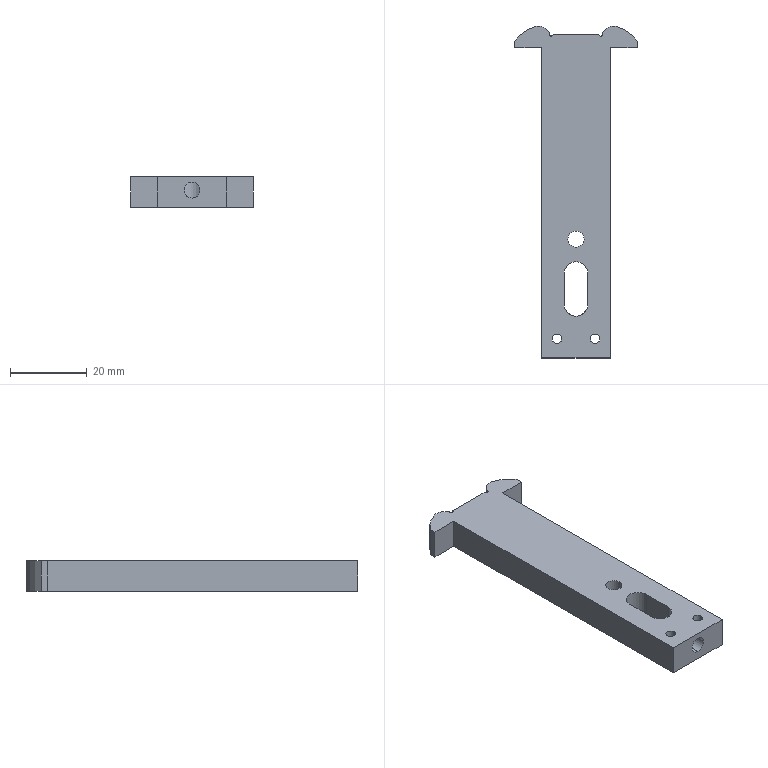Part | STEP file | BU-C07#180 | 1 solid | 31 faces | box 32 x 86.655 x 8 mm | volume 11719 mm3 | cylinder 17 | plane 14 | commonest cylinder face diameters 2.5 x4 4.2 x4 1 x3 5 x2 6.2 x2 19.8 x2